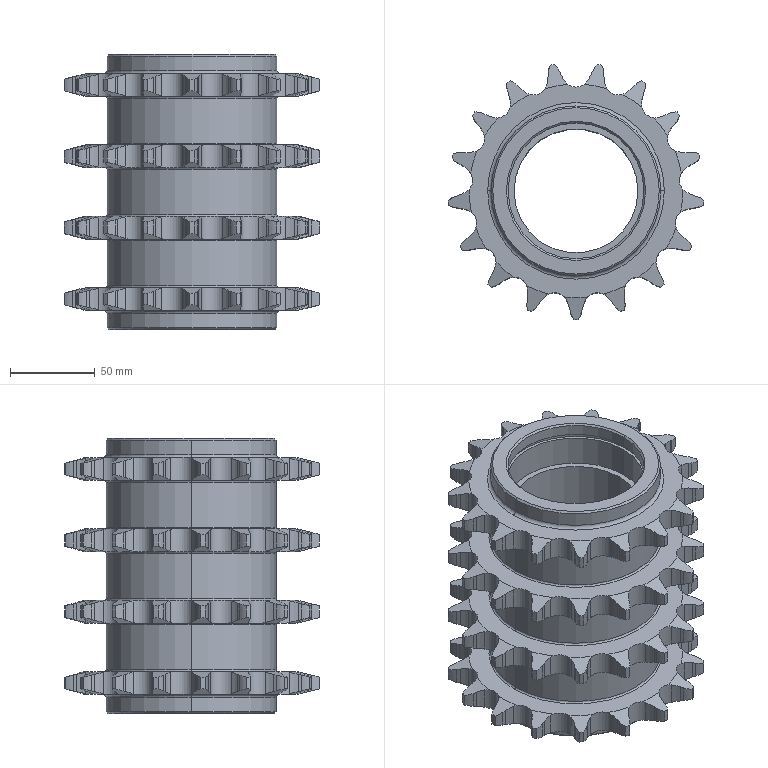Part | STEP file | 07-Sprocket | 1 solid | 752 faces | box 150.693 x 150.061 x 162 mm | volume 851897 mm3 | cylinder 432 | cone 152 | plane 152 | torus 16 | commonest cylinder face diameters 26.48 x136 41.357 x136 15.957 x68 151.118 x68 100 x10 80 x8